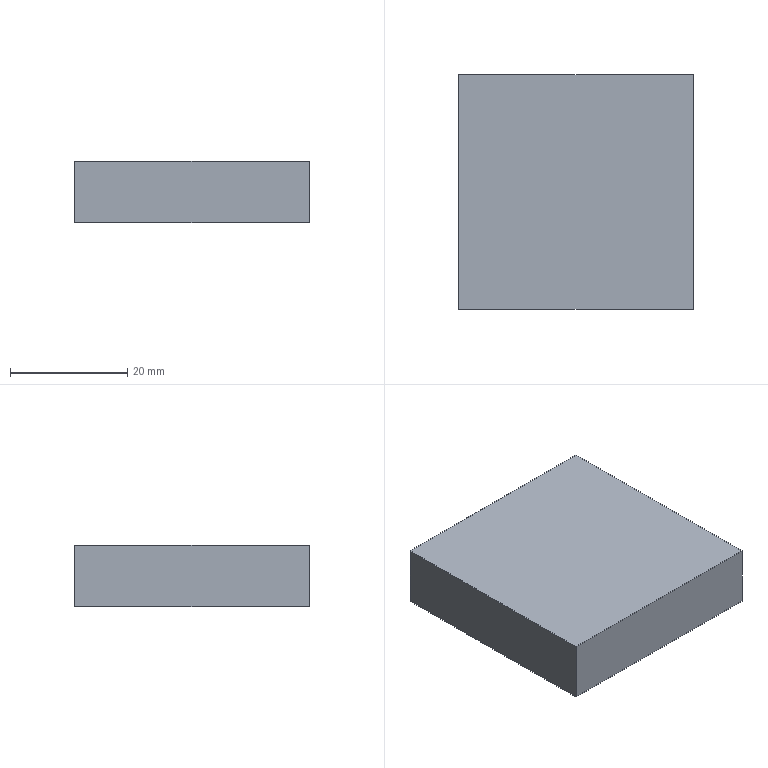Part | NX | features solid 2 | 1 solid | 6 faces | box 40 x 40 x 10.5 mm | volume 16800 mm3 | plane 6
STEP:
#1=CARTESIAN_POINT('',(-995.,-60.,-45.));
#2=VERTEX_POINT('',#1);
#3=CARTESIAN_POINT('',(-955.,-60.,-45.));
#4=VERTEX_POINT('',#3);
#5=CARTESIAN_POINT('',(-525.,-60.,-45.));
#6=DIRECTION('',(1.,0.,0.));
#7=VECTOR('',#6,1000.);
#8=LINE('',#5,#7);
#9=EDGE_CURVE('',#2,#4,#8,.T.);
#10=ORIENTED_EDGE('',*,*,#9,.T.);
#11=CARTESIAN_POINT('',(-955.,-60.,-34.5));
#12=VERTEX_POINT('',#11);
#13=CARTESIAN_POINT('',(-955.,-60.,-35.));
#14=DIRECTION('',(0.,0.,1.));
#15=VECTOR('',#14,1000.);
#16=LINE('',#13,#15);
#17=EDGE_CURVE('',#12,#4,#16,.F.);
#18=ORIENTED_EDGE('',*,*,#17,.F.);
#19=CARTESIAN_POINT('',(-995.,-60.,-34.5));
#20=VERTEX_POINT('',#19);
#21=CARTESIAN_POINT('',(-746.2,-60.,-34.5));
#22=DIRECTION('',(1.,0.,0.));
#23=VECTOR('',#22,1000.);
#24=LINE('',#21,#23);
#25=EDGE_CURVE('',#20,#12,#24,.T.);
#26=ORIENTED_EDGE('',*,*,#25,.F.);
#27=CARTESIAN_POINT('',(-995.,-60.,-35.));
#28=DIRECTION('',(0.,0.,-1.));
#29=VECTOR('',#28,1000.);
#30=LINE('',#27,#29);
#31=EDGE_CURVE('',#20,#2,#30,.T.);
#32=ORIENTED_EDGE('',*,*,#31,.T.);
#33=EDGE_LOOP('',(#10,#18,#26,#32));
#34=FACE_BOUND('',#33,.T.);
#35=CARTESIAN_POINT('',(-746.2,-60.,-35.));
#36=DIRECTION('',(0.,-1.,0.));
#37=DIRECTION('',(0.,0.,1.));
#38=AXIS2_PLACEMENT_3D('',#35,#36,#37);
#39=PLANE('',#38);
#40=ADVANCED_FACE('',(#34),#39,.T.);
#41=CARTESIAN_POINT('',(-955.,-20.,-45.));
#42=VERTEX_POINT('',#41);
#43=CARTESIAN_POINT('',(-955.,-60.,-45.));
#44=DIRECTION('',(0.,-1.,0.));
#45=VECTOR('',#44,1000.);
#46=LINE('',#43,#45);
#47=EDGE_CURVE('',#4,#42,#46,.F.);
#48=ORIENTED_EDGE('',*,*,#47,.T.);
#49=CARTESIAN_POINT('',(-955.,-20.,-34.5));
#50=VERTEX_POINT('',#49);
#51=CARTESIAN_POINT('',(-955.,-20.,-35.));
#52=DIRECTION('',(0.,0.,1.));
#53=VECTOR('',#52,1000.);
#54=LINE('',#51,#53);
#55=EDGE_CURVE('',#50,#42,#54,.F.);
#56=ORIENTED_EDGE('',*,*,#55,.F.);
#57=CARTESIAN_POINT('',(-955.,280.,-34.5));
#58=DIRECTION('',(0.,-1.,0.));
#59=VECTOR('',#58,1000.);
#60=LINE('',#57,#59);
#61=EDGE_CURVE('',#12,#50,#60,.F.);
#62=ORIENTED_EDGE('',*,*,#61,.F.);
#63=ORIENTED_EDGE('',*,*,#17,.T.);
#64=EDGE_LOOP('',(#48,#56,#62,#63));
#65=FACE_BOUND('',#64,.T.);
#66=CARTESIAN_POINT('',(-955.,280.,-35.));
#67=DIRECTION('',(-1.,0.,0.));
#68=DIRECTION('',(0.,1.,0.));
#69=AXIS2_PLACEMENT_3D('',#66,#67,#68);
#70=PLANE('',#69);
#71=ADVANCED_FACE('',(#65),#70,.F.);
#72=CARTESIAN_POINT('',(-995.,-20.,-45.));
#73=VERTEX_POINT('',#72);
#74=CARTESIAN_POINT('',(-525.,-20.,-45.));
#75=DIRECTION('',(1.,0.,0.));
#76=VECTOR('',#75,1000.);
#77=LINE('',#74,#76);
#78=EDGE_CURVE('',#73,#42,#77,.T.);
#79=ORIENTED_EDGE('',*,*,#78,.F.);
#80=CARTESIAN_POINT('',(-995.,-20.,-34.5));
#81=VERTEX_POINT('',#80);
#82=CARTESIAN_POINT('',(-995.,-20.,-35.));
#83=DIRECTION('',(0.,0.,-1.));
#84=VECTOR('',#83,1000.);
#85=LINE('',#82,#84);
#86=EDGE_CURVE('',#81,#73,#85,.T.);
#87=ORIENTED_EDGE('',*,*,#86,.F.);
#88=CARTESIAN_POINT('',(-1045.,-20.,-34.5));
#89=DIRECTION('',(1.,0.,0.));
#90=VECTOR('',#89,1000.);
#91=LINE('',#88,#90);
#92=EDGE_CURVE('',#81,#50,#91,.T.);
#93=ORIENTED_EDGE('',*,*,#92,.T.);
#94=ORIENTED_EDGE('',*,*,#55,.T.);
#95=EDGE_LOOP('',(#79,#87,#93,#94));
#96=FACE_BOUND('',#95,.T.);
#97=CARTESIAN_POINT('',(-1045.,-20.,-35.));
#98=DIRECTION('',(0.,-1.,0.));
#99=DIRECTION('',(0.,0.,1.));
#100=AXIS2_PLACEMENT_3D('',#97,#98,#99);
#101=PLANE('',#100);
#102=ADVANCED_FACE('',(#96),#101,.F.);
#103=CARTESIAN_POINT('',(-995.,-60.,-45.));
#104=DIRECTION('',(0.,1.,0.));
#105=VECTOR('',#104,1000.);
#106=LINE('',#103,#105);
#107=EDGE_CURVE('',#2,#73,#106,.T.);
#108=ORIENTED_EDGE('',*,*,#107,.F.);
#109=ORIENTED_EDGE('',*,*,#31,.F.);
#110=CARTESIAN_POINT('',(-995.,280.,-34.5));
#111=DIRECTION('',(0.,1.,0.));
#112=VECTOR('',#111,1000.);
#113=LINE('',#110,#112);
#114=EDGE_CURVE('',#20,#81,#113,.T.);
#115=ORIENTED_EDGE('',*,*,#114,.T.);
#116=ORIENTED_EDGE('',*,*,#86,.T.);
#117=EDGE_LOOP('',(#108,#109,#115,#116));
#118=FACE_BOUND('',#117,.T.);
#119=CARTESIAN_POINT('',(-995.,280.,-95.));
#120=DIRECTION('',(1.,0.,0.));
#121=DIRECTION('',(0.,-1.,0.));
#122=AXIS2_PLACEMENT_3D('',#119,#120,#121);
#123=PLANE('',#122);
#124=ADVANCED_FACE('',(#118),#123,.F.);
#125=ORIENTED_EDGE('',*,*,#25,.T.);
#126=ORIENTED_EDGE('',*,*,#61,.T.);
#127=ORIENTED_EDGE('',*,*,#92,.F.);
#128=ORIENTED_EDGE('',*,*,#114,.F.);
#129=EDGE_LOOP('',(#125,#126,#127,#128));
#130=FACE_BOUND('',#129,.T.);
#131=CARTESIAN_POINT('',(-525.,-60.,-34.5));
#132=DIRECTION('',(0.,0.,-1.));
#133=DIRECTION('',(0.,-1.,0.));
#134=AXIS2_PLACEMENT_3D('',#131,#132,#133);
#135=PLANE('',#134);
#136=ADVANCED_FACE('',(#130),#135,.F.);
#137=ORIENTED_EDGE('',*,*,#107,.T.);
#138=ORIENTED_EDGE('',*,*,#78,.T.);
#139=ORIENTED_EDGE('',*,*,#47,.F.);
#140=ORIENTED_EDGE('',*,*,#9,.F.);
#141=EDGE_LOOP('',(#137,#138,#139,#140));
#142=FACE_BOUND('',#141,.T.);
#143=CARTESIAN_POINT('',(-525.,-60.,-45.));
#144=DIRECTION('',(0.,0.,-1.));
#145=DIRECTION('',(0.,-1.,0.));
#146=AXIS2_PLACEMENT_3D('',#143,#144,#145);
#147=PLANE('',#146);
#148=ADVANCED_FACE('',(#142),#147,.T.);
#149=CLOSED_SHELL('',(#40,#71,#102,#124,#136,#148));
#150=MANIFOLD_SOLID_BREP('',#149);
#151=(LENGTH_UNIT()NAMED_UNIT(*)SI_UNIT(.MILLI.,.METRE.));
#152=UNCERTAINTY_MEASURE_WITH_UNIT(LENGTH_MEASURE(0.00001),#151,'','');
#153=(NAMED_UNIT(*)PLANE_ANGLE_UNIT()SI_UNIT($,.RADIAN.));
#154=(NAMED_UNIT(*)SI_UNIT($,.STERADIAN.)SOLID_ANGLE_UNIT());
#155=(GEOMETRIC_REPRESENTATION_CONTEXT(3)GLOBAL_UNCERTAINTY_ASSIGNED_CONTEXT((#152))GLOBAL_UNIT_ASSIGNED_CONTEXT((#151,#153,#154))REPRESENTATION_CONTEXT('',''));
#156=ADVANCED_BREP_SHAPE_REPRESENTATION('',(#150),#155);